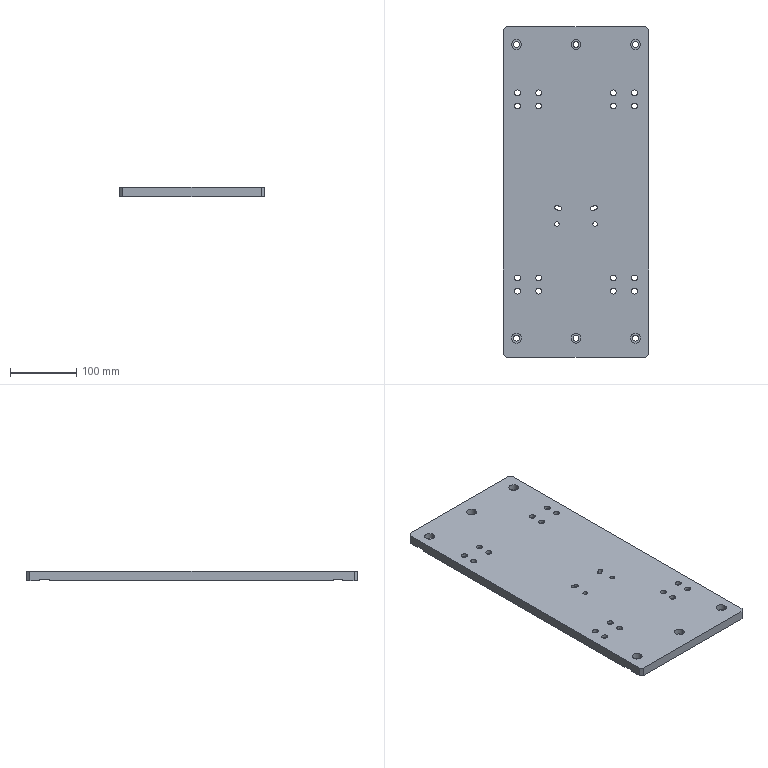Part | STEP file | fBY02F02M-00-04A | 1 solid | 138 faces | box 220 x 500 x 14 mm | volume 1483001 mm3 | cylinder 98 | plane 40 | commonest cylinder face diameters 9 x44 15 x44 6.8 x10